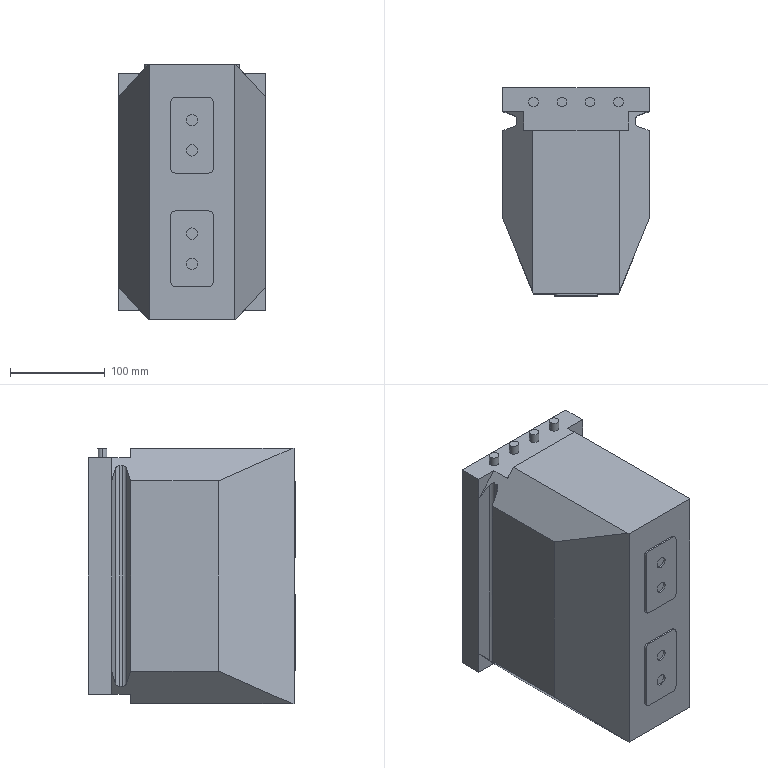Part | SolidWorks | features BaseBody 1 | 1 solid | 86 faces | box 155 x 220 x 270 mm | volume 7916684 mm3 | plane 50 | cylinder 36 | commonest cylinder face diameters 10 x28 12 x8